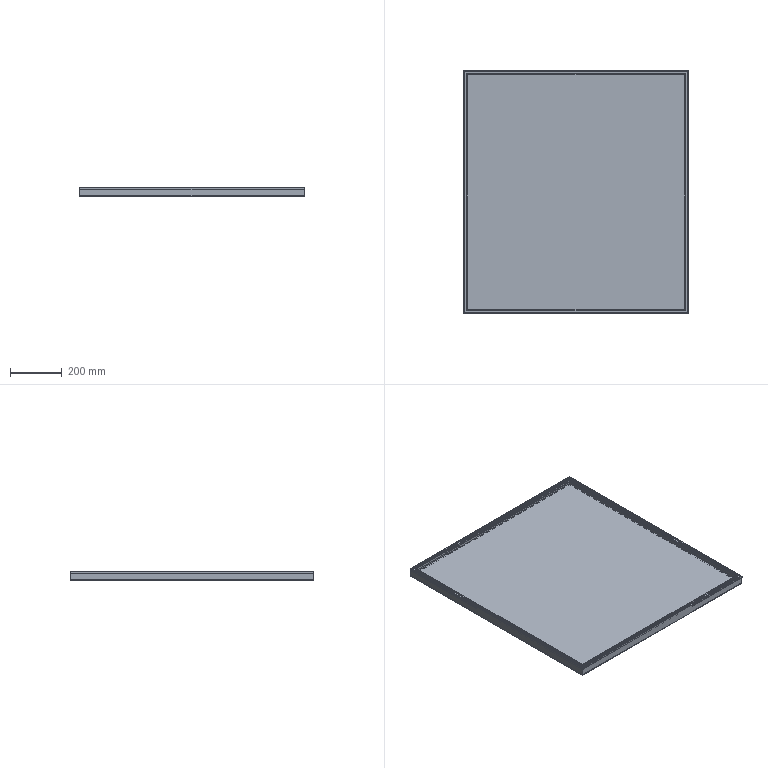Part | 5 solids | 94 faces | box 870 x 940 x 35 mm | volume 2912512 mm3 | plane 86 | cylinder 8 | commonest cylinder face diameters 1 x4 2 x4